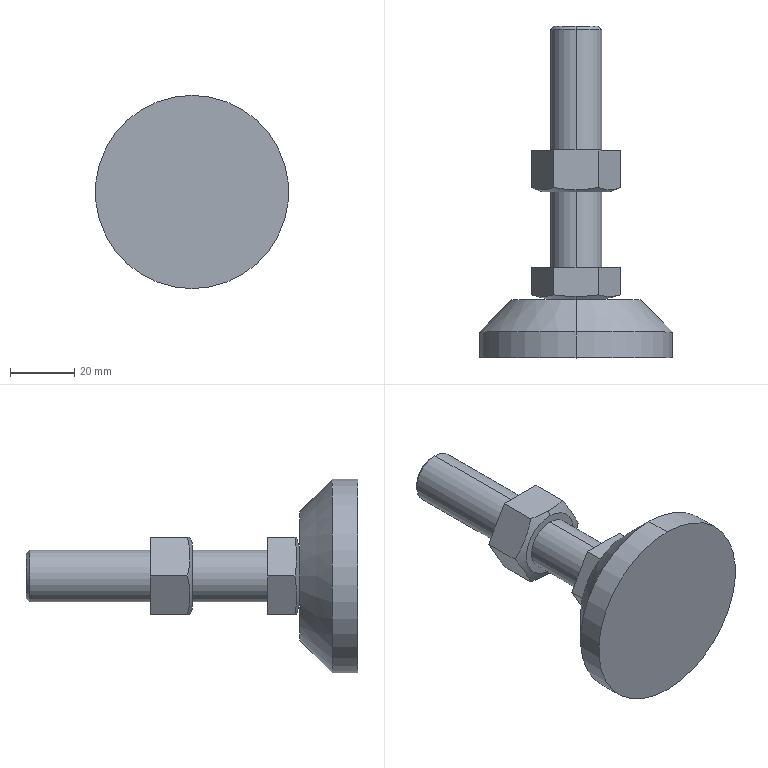Part | STEP file | PN_0021_default | 2 solids | 36 faces | box 60 x 103 x 60 mm | volume 66755 mm3 | plane 18 | cone 12 | cylinder 6 | commonest cylinder face diameters 13.835 x2 16 x2 60 x2